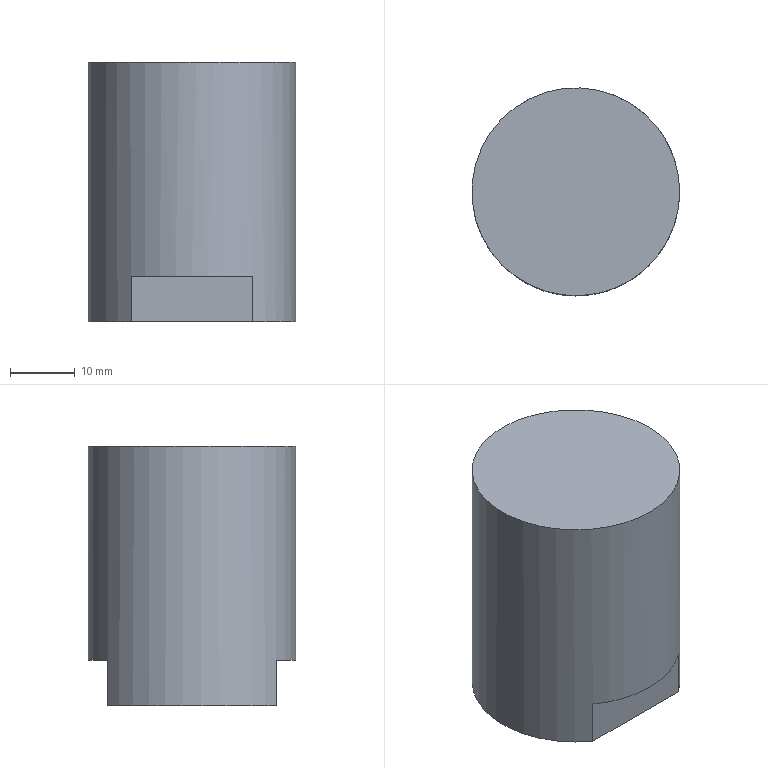Part | STEP file | CMT7E v7 | 1 solid | 7 faces | box 32 x 32 x 40 mm | volume 31637 mm3 | plane 6 | cylinder 1 | commonest cylinder face diameters 32 x1
STEP:
#1=CARTESIAN_POINT('',(0.,0.,0.));
#2=DIRECTION('',(0.,0.,1.));
#3=DIRECTION('',(1.,0.,0.));
#4=AXIS2_PLACEMENT_3D('',#1,#2,#3);
#5=CARTESIAN_POINT('',(16.,0.,99.));
#6=VERTEX_POINT('',#5);
#7=CARTESIAN_POINT('',(0.,0.,99.));
#8=DIRECTION('',(0.,0.,-1.));
#9=DIRECTION('',(1.,0.,0.));
#10=AXIS2_PLACEMENT_3D('',#7,#8,#9);
#11=CIRCLE('',#10,16.);
#12=CARTESIAN_POINT('',(0.,0.,99.));
#13=DIRECTION('',(0.,0.,-1.));
#14=DIRECTION('',(1.,0.,0.));
#15=AXIS2_PLACEMENT_3D('',#12,#13,#14);
#16=PLANE('',#15);
#17=CARTESIAN_POINT('',(0.,0.));
#18=DIRECTION('',(1.,0.));
#19=AXIS2_PLACEMENT_2D('',#17,#18);
#20=CIRCLE('',#19,16.);
#21=(GEOMETRIC_REPRESENTATION_CONTEXT(2)PARAMETRIC_REPRESENTATION_CONTEXT()REPRESENTATION_CONTEXT('',''));
#22=DEFINITIONAL_REPRESENTATION('',(#20),#21);
#23=PCURVE('',#16,#22);
#24=CARTESIAN_POINT('',(0.,0.,99.));
#25=DIRECTION('',(0.,0.,-1.));
#26=DIRECTION('',(1.,0.,0.));
#27=AXIS2_PLACEMENT_3D('',#24,#25,#26);
#28=CYLINDRICAL_SURFACE('',#27,16.);
#29=CARTESIAN_POINT('',(0.,0.));
#30=DIRECTION('',(1.,0.));
#31=VECTOR('',#30,1.);
#32=LINE('',#29,#31);
#33=(GEOMETRIC_REPRESENTATION_CONTEXT(2)PARAMETRIC_REPRESENTATION_CONTEXT()REPRESENTATION_CONTEXT('',''));
#34=DEFINITIONAL_REPRESENTATION('',(#32),#33);
#35=PCURVE('',#28,#34);
#36=SURFACE_CURVE('',#11,(#23,#35),.PCURVE_S1.);
#37=EDGE_CURVE('',#6,#6,#36,.T.);
#38=ORIENTED_EDGE('',*,*,#37,.F.);
#39=EDGE_LOOP('',(#38));
#40=FACE_BOUND('',#39,.T.);
#41=ADVANCED_FACE('',(#40),#16,.F.);
#42=CARTESIAN_POINT('',(9.327,-13.,59.));
#43=VERTEX_POINT('',#42);
#44=CARTESIAN_POINT('',(-9.327,-13.,59.));
#45=VERTEX_POINT('',#44);
#46=CARTESIAN_POINT('',(8.25,-13.,59.));
#47=DIRECTION('',(-1.,0.,0.));
#48=VECTOR('',#47,1.);
#49=LINE('',#46,#48);
#50=CARTESIAN_POINT('',(0.,0.,59.));
#51=DIRECTION('',(0.,0.,-1.));
#52=DIRECTION('',(1.,0.,0.));
#53=AXIS2_PLACEMENT_3D('',#50,#51,#52);
#54=PLANE('',#53);
#55=CARTESIAN_POINT('',(8.25,13.));
#56=DIRECTION('',(-1.,0.));
#57=VECTOR('',#56,1.);
#58=LINE('',#55,#57);
#59=(GEOMETRIC_REPRESENTATION_CONTEXT(2)PARAMETRIC_REPRESENTATION_CONTEXT()REPRESENTATION_CONTEXT('',''));
#60=DEFINITIONAL_REPRESENTATION('',(#58),#59);
#61=PCURVE('',#54,#60);
#62=CARTESIAN_POINT('',(16.5,-13.,59.));
#63=DIRECTION('',(0.,1.,0.));
#64=DIRECTION('',(-1.,0.,0.));
#65=AXIS2_PLACEMENT_3D('',#62,#63,#64);
#66=PLANE('',#65);
#67=CARTESIAN_POINT('',(8.25,0.));
#68=DIRECTION('',(1.,0.));
#69=VECTOR('',#68,1.);
#70=LINE('',#67,#69);
#71=(GEOMETRIC_REPRESENTATION_CONTEXT(2)PARAMETRIC_REPRESENTATION_CONTEXT()REPRESENTATION_CONTEXT('',''));
#72=DEFINITIONAL_REPRESENTATION('',(#70),#71);
#73=PCURVE('',#66,#72);
#74=SURFACE_CURVE('',#49,(#61,#73),.PCURVE_S1.);
#75=EDGE_CURVE('',#43,#45,#74,.T.);
#76=ORIENTED_EDGE('',*,*,#75,.T.);
#77=CARTESIAN_POINT('',(-9.327,13.,59.));
#78=VERTEX_POINT('',#77);
#79=CARTESIAN_POINT('',(0.,0.,59.));
#80=DIRECTION('',(0.,0.,-1.));
#81=DIRECTION('',(1.,0.,0.));
#82=AXIS2_PLACEMENT_3D('',#79,#80,#81);
#83=CIRCLE('',#82,16.);
#84=CARTESIAN_POINT('',(0.,0.));
#85=DIRECTION('',(1.,0.));
#86=AXIS2_PLACEMENT_2D('',#84,#85);
#87=CIRCLE('',#86,16.);
#88=(GEOMETRIC_REPRESENTATION_CONTEXT(2)PARAMETRIC_REPRESENTATION_CONTEXT()REPRESENTATION_CONTEXT('',''));
#89=DEFINITIONAL_REPRESENTATION('',(#87),#88);
#90=PCURVE('',#54,#89);
#91=CARTESIAN_POINT('',(0.,40.));
#92=DIRECTION('',(1.,0.));
#93=VECTOR('',#92,1.);
#94=LINE('',#91,#93);
#95=(GEOMETRIC_REPRESENTATION_CONTEXT(2)PARAMETRIC_REPRESENTATION_CONTEXT()REPRESENTATION_CONTEXT('',''));
#96=DEFINITIONAL_REPRESENTATION('',(#94),#95);
#97=PCURVE('',#28,#96);
#98=SURFACE_CURVE('',#83,(#90,#97),.PCURVE_S1.);
#99=EDGE_CURVE('',#45,#78,#98,.T.);
#100=ORIENTED_EDGE('',*,*,#99,.T.);
#101=CARTESIAN_POINT('',(9.327,13.,59.));
#102=VERTEX_POINT('',#101);
#103=CARTESIAN_POINT('',(-8.25,13.,59.));
#104=DIRECTION('',(1.,0.,0.));
#105=VECTOR('',#104,1.);
#106=LINE('',#103,#105);
#107=CARTESIAN_POINT('',(-8.25,-13.));
#108=DIRECTION('',(1.,0.));
#109=VECTOR('',#108,1.);
#110=LINE('',#107,#109);
#111=(GEOMETRIC_REPRESENTATION_CONTEXT(2)PARAMETRIC_REPRESENTATION_CONTEXT()REPRESENTATION_CONTEXT('',''));
#112=DEFINITIONAL_REPRESENTATION('',(#110),#111);
#113=PCURVE('',#54,#112);
#114=CARTESIAN_POINT('',(-16.5,13.,59.));
#115=DIRECTION('',(0.,-1.,0.));
#116=DIRECTION('',(1.,0.,0.));
#117=AXIS2_PLACEMENT_3D('',#114,#115,#116);
#118=PLANE('',#117);
#119=CARTESIAN_POINT('',(8.25,0.));
#120=DIRECTION('',(1.,0.));
#121=VECTOR('',#120,1.);
#122=LINE('',#119,#121);
#123=(GEOMETRIC_REPRESENTATION_CONTEXT(2)PARAMETRIC_REPRESENTATION_CONTEXT()REPRESENTATION_CONTEXT('',''));
#124=DEFINITIONAL_REPRESENTATION('',(#122),#123);
#125=PCURVE('',#118,#124);
#126=SURFACE_CURVE('',#106,(#113,#125),.PCURVE_S1.);
#127=EDGE_CURVE('',#78,#102,#126,.T.);
#128=ORIENTED_EDGE('',*,*,#127,.T.);
#129=CARTESIAN_POINT('',(16.,0.,59.));
#130=VERTEX_POINT('',#129);
#131=CARTESIAN_POINT('',(0.,0.,59.));
#132=DIRECTION('',(0.,0.,-1.));
#133=DIRECTION('',(1.,0.,0.));
#134=AXIS2_PLACEMENT_3D('',#131,#132,#133);
#135=CIRCLE('',#134,16.);
#136=CARTESIAN_POINT('',(0.,0.));
#137=DIRECTION('',(1.,0.));
#138=AXIS2_PLACEMENT_2D('',#136,#137);
#139=CIRCLE('',#138,16.);
#140=(GEOMETRIC_REPRESENTATION_CONTEXT(2)PARAMETRIC_REPRESENTATION_CONTEXT()REPRESENTATION_CONTEXT('',''));
#141=DEFINITIONAL_REPRESENTATION('',(#139),#140);
#142=PCURVE('',#54,#141);
#143=CARTESIAN_POINT('',(0.,40.));
#144=DIRECTION('',(1.,0.));
#145=VECTOR('',#144,1.);
#146=LINE('',#143,#145);
#147=(GEOMETRIC_REPRESENTATION_CONTEXT(2)PARAMETRIC_REPRESENTATION_CONTEXT()REPRESENTATION_CONTEXT('',''));
#148=DEFINITIONAL_REPRESENTATION('',(#146),#147);
#149=PCURVE('',#28,#148);
#150=SURFACE_CURVE('',#135,(#142,#149),.PCURVE_S1.);
#151=EDGE_CURVE('',#102,#130,#150,.T.);
#152=ORIENTED_EDGE('',*,*,#151,.T.);
#153=CARTESIAN_POINT('',(0.,0.,59.));
#154=DIRECTION('',(0.,0.,-1.));
#155=DIRECTION('',(1.,0.,0.));
#156=AXIS2_PLACEMENT_3D('',#153,#154,#155);
#157=CIRCLE('',#156,16.);
#158=CARTESIAN_POINT('',(0.,0.));
#159=DIRECTION('',(1.,0.));
#160=AXIS2_PLACEMENT_2D('',#158,#159);
#161=CIRCLE('',#160,16.);
#162=(GEOMETRIC_REPRESENTATION_CONTEXT(2)PARAMETRIC_REPRESENTATION_CONTEXT()REPRESENTATION_CONTEXT('',''));
#163=DEFINITIONAL_REPRESENTATION('',(#161),#162);
#164=PCURVE('',#54,#163);
#165=CARTESIAN_POINT('',(0.,40.));
#166=DIRECTION('',(1.,0.));
#167=VECTOR('',#166,1.);
#168=LINE('',#165,#167);
#169=(GEOMETRIC_REPRESENTATION_CONTEXT(2)PARAMETRIC_REPRESENTATION_CONTEXT()REPRESENTATION_CONTEXT('',''));
#170=DEFINITIONAL_REPRESENTATION('',(#168),#169);
#171=PCURVE('',#28,#170);
#172=SURFACE_CURVE('',#157,(#164,#171),.PCURVE_S1.);
#173=EDGE_CURVE('',#130,#43,#172,.T.);
#174=ORIENTED_EDGE('',*,*,#173,.T.);
#175=EDGE_LOOP('',(#76,#100,#128,#152,#174));
#176=FACE_BOUND('',#175,.T.);
#177=ADVANCED_FACE('',(#176),#54,.T.);
#178=ORIENTED_EDGE('',*,*,#37,.T.);
#179=CARTESIAN_POINT('',(16.,0.,99.));
#180=CARTESIAN_POINT('',(16.,0.,59.));
#181=B_SPLINE_CURVE_WITH_KNOTS('',1,(#179,#180),.UNSPECIFIED.,.F.,.F.,(2,2),(0.,40.),.PIECEWISE_BEZIER_KNOTS.);
#182=CARTESIAN_POINT('',(6.283,0.));
#183=DIRECTION('',(0.,1.));
#184=VECTOR('',#183,1.);
#185=LINE('',#182,#184);
#186=(GEOMETRIC_REPRESENTATION_CONTEXT(2)PARAMETRIC_REPRESENTATION_CONTEXT()REPRESENTATION_CONTEXT('',''));
#187=DEFINITIONAL_REPRESENTATION('',(#185),#186);
#188=PCURVE('',#28,#187);
#189=CARTESIAN_POINT('',(0.,0.));
#190=DIRECTION('',(0.,1.));
#191=VECTOR('',#190,1.);
#192=LINE('',#189,#191);
#193=(GEOMETRIC_REPRESENTATION_CONTEXT(2)PARAMETRIC_REPRESENTATION_CONTEXT()REPRESENTATION_CONTEXT('',''));
#194=DEFINITIONAL_REPRESENTATION('',(#192),#193);
#195=PCURVE('',#28,#194);
#196=SEAM_CURVE('',#181,(#188,#195),.PCURVE_S1.);
#197=EDGE_CURVE('',#6,#130,#196,.T.);
#198=ORIENTED_EDGE('',*,*,#197,.T.);
#199=ORIENTED_EDGE('',*,*,#151,.F.);
#200=CARTESIAN_POINT('',(9.327,13.,66.));
#201=VERTEX_POINT('',#200);
#202=CARTESIAN_POINT('',(9.327,13.,99.));
#203=DIRECTION('',(0.,0.,1.));
#204=VECTOR('',#203,1.);
#205=LINE('',#202,#204);
#206=CARTESIAN_POINT('',(5.335,0.));
#207=DIRECTION('',(0.,-1.));
#208=VECTOR('',#207,1.);
#209=LINE('',#206,#208);
#210=(GEOMETRIC_REPRESENTATION_CONTEXT(2)PARAMETRIC_REPRESENTATION_CONTEXT()REPRESENTATION_CONTEXT('',''));
#211=DEFINITIONAL_REPRESENTATION('',(#209),#210);
#212=PCURVE('',#28,#211);
#213=CARTESIAN_POINT('',(25.827,40.));
#214=DIRECTION('',(0.,1.));
#215=VECTOR('',#214,1.);
#216=LINE('',#213,#215);
#217=(GEOMETRIC_REPRESENTATION_CONTEXT(2)PARAMETRIC_REPRESENTATION_CONTEXT()REPRESENTATION_CONTEXT('',''));
#218=DEFINITIONAL_REPRESENTATION('',(#216),#217);
#219=PCURVE('',#118,#218);
#220=SURFACE_CURVE('',#205,(#212,#219),.PCURVE_S1.);
#221=EDGE_CURVE('',#102,#201,#220,.T.);
#222=ORIENTED_EDGE('',*,*,#221,.T.);
#223=CARTESIAN_POINT('',(-9.327,13.,66.));
#224=VERTEX_POINT('',#223);
#225=CARTESIAN_POINT('',(0.,0.,66.));
#226=DIRECTION('',(0.,0.,1.));
#227=DIRECTION('',(1.,0.,0.));
#228=AXIS2_PLACEMENT_3D('',#225,#226,#227);
#229=CIRCLE('',#228,16.);
#230=CARTESIAN_POINT('',(6.283,33.));
#231=DIRECTION('',(-1.,0.));
#232=VECTOR('',#231,1.);
#233=LINE('',#230,#232);
#234=(GEOMETRIC_REPRESENTATION_CONTEXT(2)PARAMETRIC_REPRESENTATION_CONTEXT()REPRESENTATION_CONTEXT('',''));
#235=DEFINITIONAL_REPRESENTATION('',(#233),#234);
#236=PCURVE('',#28,#235);
#237=CARTESIAN_POINT('',(0.,15.5,66.));
#238=DIRECTION('',(0.,0.,1.));
#239=DIRECTION('',(1.,0.,0.));
#240=AXIS2_PLACEMENT_3D('',#237,#238,#239);
#241=PLANE('',#240);
#242=CARTESIAN_POINT('',(0.,-15.5));
#243=DIRECTION('',(1.,0.));
#244=AXIS2_PLACEMENT_2D('',#242,#243);
#245=CIRCLE('',#244,16.);
#246=(GEOMETRIC_REPRESENTATION_CONTEXT(2)PARAMETRIC_REPRESENTATION_CONTEXT()REPRESENTATION_CONTEXT('',''));
#247=DEFINITIONAL_REPRESENTATION('',(#245),#246);
#248=PCURVE('',#241,#247);
#249=SURFACE_CURVE('',#229,(#236,#248),.PCURVE_S1.);
#250=EDGE_CURVE('',#201,#224,#249,.T.);
#251=ORIENTED_EDGE('',*,*,#250,.T.);
#252=CARTESIAN_POINT('',(-9.327,13.,99.));
#253=DIRECTION('',(0.,0.,-1.));
#254=VECTOR('',#253,1.);
#255=LINE('',#252,#254);
#256=CARTESIAN_POINT('',(4.09,0.));
#257=DIRECTION('',(0.,1.));
#258=VECTOR('',#257,1.);
#259=LINE('',#256,#258);
#260=(GEOMETRIC_REPRESENTATION_CONTEXT(2)PARAMETRIC_REPRESENTATION_CONTEXT()REPRESENTATION_CONTEXT('',''));
#261=DEFINITIONAL_REPRESENTATION('',(#259),#260);
#262=PCURVE('',#28,#261);
#263=CARTESIAN_POINT('',(7.173,40.));
#264=DIRECTION('',(0.,-1.));
#265=VECTOR('',#264,1.);
#266=LINE('',#263,#265);
#267=(GEOMETRIC_REPRESENTATION_CONTEXT(2)PARAMETRIC_REPRESENTATION_CONTEXT()REPRESENTATION_CONTEXT('',''));
#268=DEFINITIONAL_REPRESENTATION('',(#266),#267);
#269=PCURVE('',#118,#268);
#270=SURFACE_CURVE('',#255,(#262,#269),.PCURVE_S1.);
#271=EDGE_CURVE('',#224,#78,#270,.T.);
#272=ORIENTED_EDGE('',*,*,#271,.T.);
#273=ORIENTED_EDGE('',*,*,#99,.F.);
#274=CARTESIAN_POINT('',(-9.327,-13.,66.));
#275=VERTEX_POINT('',#274);
#276=CARTESIAN_POINT('',(-9.327,-13.,99.));
#277=DIRECTION('',(0.,0.,1.));
#278=VECTOR('',#277,1.);
#279=LINE('',#276,#278);
#280=CARTESIAN_POINT('',(2.193,0.));
#281=DIRECTION('',(0.,-1.));
#282=VECTOR('',#281,1.);
#283=LINE('',#280,#282);
#284=(GEOMETRIC_REPRESENTATION_CONTEXT(2)PARAMETRIC_REPRESENTATION_CONTEXT()REPRESENTATION_CONTEXT('',''));
#285=DEFINITIONAL_REPRESENTATION('',(#283),#284);
#286=PCURVE('',#28,#285);
#287=CARTESIAN_POINT('',(25.827,40.));
#288=DIRECTION('',(0.,1.));
#289=VECTOR('',#288,1.);
#290=LINE('',#287,#289);
#291=(GEOMETRIC_REPRESENTATION_CONTEXT(2)PARAMETRIC_REPRESENTATION_CONTEXT()REPRESENTATION_CONTEXT('',''));
#292=DEFINITIONAL_REPRESENTATION('',(#290),#291);
#293=PCURVE('',#66,#292);
#294=SURFACE_CURVE('',#279,(#286,#293),.PCURVE_S1.);
#295=EDGE_CURVE('',#45,#275,#294,.T.);
#296=ORIENTED_EDGE('',*,*,#295,.T.);
#297=CARTESIAN_POINT('',(9.327,-13.,66.));
#298=VERTEX_POINT('',#297);
#299=CARTESIAN_POINT('',(0.,0.,66.));
#300=DIRECTION('',(0.,0.,1.));
#301=DIRECTION('',(1.,0.,0.));
#302=AXIS2_PLACEMENT_3D('',#299,#300,#301);
#303=CIRCLE('',#302,16.);
#304=CARTESIAN_POINT('',(6.283,33.));
#305=DIRECTION('',(-1.,0.));
#306=VECTOR('',#305,1.);
#307=LINE('',#304,#306);
#308=(GEOMETRIC_REPRESENTATION_CONTEXT(2)PARAMETRIC_REPRESENTATION_CONTEXT()REPRESENTATION_CONTEXT('',''));
#309=DEFINITIONAL_REPRESENTATION('',(#307),#308);
#310=PCURVE('',#28,#309);
#311=CARTESIAN_POINT('',(0.,-15.5,66.));
#312=DIRECTION('',(0.,0.,1.));
#313=DIRECTION('',(1.,0.,0.));
#314=AXIS2_PLACEMENT_3D('',#311,#312,#313);
#315=PLANE('',#314);
#316=CARTESIAN_POINT('',(0.,15.5));
#317=DIRECTION('',(1.,0.));
#318=AXIS2_PLACEMENT_2D('',#316,#317);
#319=CIRCLE('',#318,16.);
#320=(GEOMETRIC_REPRESENTATION_CONTEXT(2)PARAMETRIC_REPRESENTATION_CONTEXT()REPRESENTATION_CONTEXT('',''));
#321=DEFINITIONAL_REPRESENTATION('',(#319),#320);
#322=PCURVE('',#315,#321);
#323=SURFACE_CURVE('',#303,(#310,#322),.PCURVE_S1.);
#324=EDGE_CURVE('',#275,#298,#323,.T.);
#325=ORIENTED_EDGE('',*,*,#324,.T.);
#326=CARTESIAN_POINT('',(9.327,-13.,99.));
#327=DIRECTION('',(0.,0.,-1.));
#328=VECTOR('',#327,1.);
#329=LINE('',#326,#328);
#330=CARTESIAN_POINT('',(0.9484,0.));
#331=DIRECTION('',(0.,1.));
#332=VECTOR('',#331,1.);
#333=LINE('',#330,#332);
#334=(GEOMETRIC_REPRESENTATION_CONTEXT(2)PARAMETRIC_REPRESENTATION_CONTEXT()REPRESENTATION_CONTEXT('',''));
#335=DEFINITIONAL_REPRESENTATION('',(#333),#334);
#336=PCURVE('',#28,#335);
#337=CARTESIAN_POINT('',(7.173,40.));
#338=DIRECTION('',(0.,-1.));
#339=VECTOR('',#338,1.);
#340=LINE('',#337,#339);
#341=(GEOMETRIC_REPRESENTATION_CONTEXT(2)PARAMETRIC_REPRESENTATION_CONTEXT()REPRESENTATION_CONTEXT('',''));
#342=DEFINITIONAL_REPRESENTATION('',(#340),#341);
#343=PCURVE('',#66,#342);
#344=SURFACE_CURVE('',#329,(#336,#343),.PCURVE_S1.);
#345=EDGE_CURVE('',#298,#43,#344,.T.);
#346=ORIENTED_EDGE('',*,*,#345,.T.);
#347=ORIENTED_EDGE('',*,*,#173,.F.);
#348=ORIENTED_EDGE('',*,*,#197,.F.);
#349=EDGE_LOOP('',(#178,#198,#199,#222,#251,#272,#273,#296,#325,#346,#347,#348));
#350=FACE_BOUND('',#349,.T.);
#351=ADVANCED_FACE('',(#350),#28,.T.);
#352=ORIENTED_EDGE('',*,*,#221,.F.);
#353=ORIENTED_EDGE('',*,*,#127,.F.);
#354=ORIENTED_EDGE('',*,*,#271,.F.);
#355=CARTESIAN_POINT('',(16.5,13.,66.));
#356=DIRECTION('',(1.,0.,0.));
#357=VECTOR('',#356,1.);
#358=LINE('',#355,#357);
#359=CARTESIAN_POINT('',(33.,7.));
#360=DIRECTION('',(1.,0.));
#361=VECTOR('',#360,1.);
#362=LINE('',#359,#361);
#363=(GEOMETRIC_REPRESENTATION_CONTEXT(2)PARAMETRIC_REPRESENTATION_CONTEXT()REPRESENTATION_CONTEXT('',''));
#364=DEFINITIONAL_REPRESENTATION('',(#362),#363);
#365=PCURVE('',#118,#364);
#366=CARTESIAN_POINT('',(16.5,-2.5));
#367=DIRECTION('',(1.,0.));
#368=VECTOR('',#367,1.);
#369=LINE('',#366,#368);
#370=(GEOMETRIC_REPRESENTATION_CONTEXT(2)PARAMETRIC_REPRESENTATION_CONTEXT()REPRESENTATION_CONTEXT('',''));
#371=DEFINITIONAL_REPRESENTATION('',(#369),#370);
#372=PCURVE('',#241,#371);
#373=SURFACE_CURVE('',#358,(#365,#372),.PCURVE_S1.);
#374=EDGE_CURVE('',#224,#201,#373,.T.);
#375=ORIENTED_EDGE('',*,*,#374,.T.);
#376=EDGE_LOOP('',(#352,#353,#354,#375));
#377=FACE_BOUND('',#376,.T.);
#378=ADVANCED_FACE('',(#377),#118,.F.);
#379=ORIENTED_EDGE('',*,*,#250,.F.);
#380=ORIENTED_EDGE('',*,*,#374,.F.);
#381=EDGE_LOOP('',(#379,#380));
#382=FACE_BOUND('',#381,.T.);
#383=ADVANCED_FACE('',(#382),#241,.F.);
#384=ORIENTED_EDGE('',*,*,#295,.F.);
#385=ORIENTED_EDGE('',*,*,#75,.F.);
#386=ORIENTED_EDGE('',*,*,#345,.F.);
#387=CARTESIAN_POINT('',(16.5,-13.,66.));
#388=DIRECTION('',(-1.,0.,0.));
#389=VECTOR('',#388,1.);
#390=LINE('',#387,#389);
#391=CARTESIAN_POINT('',(0.,7.));
#392=DIRECTION('',(1.,0.));
#393=VECTOR('',#392,1.);
#394=LINE('',#391,#393);
#395=(GEOMETRIC_REPRESENTATION_CONTEXT(2)PARAMETRIC_REPRESENTATION_CONTEXT()REPRESENTATION_CONTEXT('',''));
#396=DEFINITIONAL_REPRESENTATION('',(#394),#395);
#397=PCURVE('',#66,#396);
#398=CARTESIAN_POINT('',(16.5,2.5));
#399=DIRECTION('',(-1.,0.));
#400=VECTOR('',#399,1.);
#401=LINE('',#398,#400);
#402=(GEOMETRIC_REPRESENTATION_CONTEXT(2)PARAMETRIC_REPRESENTATION_CONTEXT()REPRESENTATION_CONTEXT('',''));
#403=DEFINITIONAL_REPRESENTATION('',(#401),#402);
#404=PCURVE('',#315,#403);
#405=SURFACE_CURVE('',#390,(#397,#404),.PCURVE_S1.);
#406=EDGE_CURVE('',#298,#275,#405,.T.);
#407=ORIENTED_EDGE('',*,*,#406,.T.);
#408=EDGE_LOOP('',(#384,#385,#386,#407));
#409=FACE_BOUND('',#408,.T.);
#410=ADVANCED_FACE('',(#409),#66,.F.);
#411=ORIENTED_EDGE('',*,*,#324,.F.);
#412=ORIENTED_EDGE('',*,*,#406,.F.);
#413=EDGE_LOOP('',(#411,#412));
#414=FACE_BOUND('',#413,.T.);
#415=ADVANCED_FACE('',(#414),#315,.F.);
#416=CLOSED_SHELL('',(#41,#177,#351,#378,#383,#410,#415));
#417=MANIFOLD_SOLID_BREP('',#416);
#418=(LENGTH_UNIT()NAMED_UNIT(*)SI_UNIT(.MILLI.,.METRE.));
#419=UNCERTAINTY_MEASURE_WITH_UNIT(LENGTH_MEASURE(0.0000001),#418,'','');
#420=(NAMED_UNIT(*)PLANE_ANGLE_UNIT()SI_UNIT($,.RADIAN.));
#421=(NAMED_UNIT(*)SI_UNIT($,.STERADIAN.)SOLID_ANGLE_UNIT());
#422=(GEOMETRIC_REPRESENTATION_CONTEXT(3)GLOBAL_UNCERTAINTY_ASSIGNED_CONTEXT((#419))GLOBAL_UNIT_ASSIGNED_CONTEXT((#418,#420,#421))REPRESENTATION_CONTEXT('',''));
#423=ADVANCED_BREP_SHAPE_REPRESENTATION('',(#4,#417),#422);